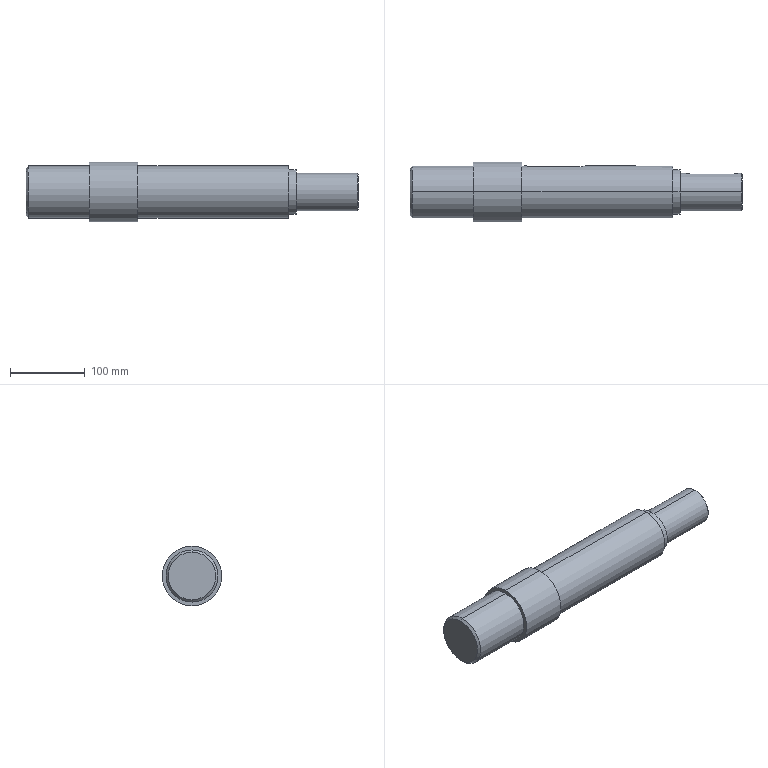Part | SolidWorks | features ICE 6, Chamfer 2, 3DProfileFeature 1, Extrusion 1, RefAxis 1 | 1 solid | 30 faces | box 445 x 80 x 80 mm | volume 1605911 mm3 | cylinder 14 | plane 12 | cone 4 | commonest cylinder face diameters 70 x4 14 x2 20 x2 50 x2 60 x2 80 x2
STEP:
#1=CARTESIAN_POINT('',(360.,0.,-24.));
#2=VERTEX_POINT('',#1);
#3=CARTESIAN_POINT('',(360.,0.,24.));
#4=VERTEX_POINT('',#3);
#5=CARTESIAN_POINT('',(360.,0.,0.));
#6=DIRECTION('',(1.,0.,0.));
#7=DIRECTION('',(0.,0.,-1.));
#8=AXIS2_PLACEMENT_3D('',#5,#6,#7);
#9=CIRCLE('',#8,24.);
#10=EDGE_CURVE('',#2,#4,#9,.T.);
#11=ORIENTED_EDGE('',*,*,#10,.F.);
#12=CARTESIAN_POINT('',(359.,0.,-25.));
#13=VERTEX_POINT('',#12);
#14=CARTESIAN_POINT('',(360.,0.,-24.));
#15=DIRECTION('',(-0.7071,0.,-0.7071));
#16=VECTOR('',#15,1000.);
#17=LINE('',#14,#16);
#18=EDGE_CURVE('',#2,#13,#17,.T.);
#19=ORIENTED_EDGE('',*,*,#18,.T.);
#20=CARTESIAN_POINT('',(359.,0.,25.));
#21=VERTEX_POINT('',#20);
#22=CARTESIAN_POINT('',(359.,0.,0.));
#23=DIRECTION('',(-1.,0.,0.));
#24=DIRECTION('',(0.,0.,-1.));
#25=AXIS2_PLACEMENT_3D('',#22,#23,#24);
#26=CIRCLE('',#25,25.);
#27=EDGE_CURVE('',#21,#13,#26,.T.);
#28=ORIENTED_EDGE('',*,*,#27,.F.);
#29=CARTESIAN_POINT('',(360.,0.,24.));
#30=DIRECTION('',(-0.7071,0.,0.7071));
#31=VECTOR('',#30,1000.);
#32=LINE('',#29,#31);
#33=EDGE_CURVE('',#4,#21,#32,.T.);
#34=ORIENTED_EDGE('',*,*,#33,.F.);
#35=EDGE_LOOP('',(#11,#19,#28,#34));
#36=FACE_OUTER_BOUND('',#35,.T.);
#37=CARTESIAN_POINT('',(360.,0.,0.));
#38=DIRECTION('',(-1.,0.,0.));
#39=DIRECTION('',(0.,0.,1.));
#40=AXIS2_PLACEMENT_3D('',#37,#38,#39);
#41=CONICAL_SURFACE('',#40,24.,0.7854);
#42=ADVANCED_FACE('',(#36),#41,.T.);
#43=CARTESIAN_POINT('',(277.,0.,-30.));
#44=VERTEX_POINT('',#43);
#45=CARTESIAN_POINT('',(277.,0.,30.));
#46=VERTEX_POINT('',#45);
#47=CARTESIAN_POINT('',(277.,0.,0.));
#48=DIRECTION('',(1.,0.,0.));
#49=DIRECTION('',(0.,0.,-1.));
#50=AXIS2_PLACEMENT_3D('',#47,#48,#49);
#51=CIRCLE('',#50,30.);
#52=EDGE_CURVE('',#44,#46,#51,.T.);
#53=ORIENTED_EDGE('',*,*,#52,.F.);
#54=CARTESIAN_POINT('',(267.,0.,-30.));
#55=VERTEX_POINT('',#54);
#56=CARTESIAN_POINT('',(277.,0.,-30.));
#57=DIRECTION('',(-1.,0.,0.));
#58=VECTOR('',#57,1000.);
#59=LINE('',#56,#58);
#60=EDGE_CURVE('',#44,#55,#59,.T.);
#61=ORIENTED_EDGE('',*,*,#60,.T.);
#62=CARTESIAN_POINT('',(267.,0.,30.));
#63=VERTEX_POINT('',#62);
#64=CARTESIAN_POINT('',(267.,0.,0.));
#65=DIRECTION('',(1.,0.,0.));
#66=DIRECTION('',(0.,0.,-1.));
#67=AXIS2_PLACEMENT_3D('',#64,#65,#66);
#68=CIRCLE('',#67,30.);
#69=EDGE_CURVE('',#55,#63,#68,.T.);
#70=ORIENTED_EDGE('',*,*,#69,.T.);
#71=CARTESIAN_POINT('',(277.,0.,30.));
#72=DIRECTION('',(-1.,0.,0.));
#73=VECTOR('',#72,1000.);
#74=LINE('',#71,#73);
#75=EDGE_CURVE('',#46,#63,#74,.T.);
#76=ORIENTED_EDGE('',*,*,#75,.F.);
#77=EDGE_LOOP('',(#53,#61,#70,#76));
#78=FACE_OUTER_BOUND('',#77,.T.);
#79=CARTESIAN_POINT('',(277.,0.,0.));
#80=DIRECTION('',(-1.,0.,0.));
#81=DIRECTION('',(0.,0.,1.));
#82=AXIS2_PLACEMENT_3D('',#79,#80,#81);
#83=CYLINDRICAL_SURFACE('',#82,30.);
#84=ADVANCED_FACE('',(#78),#83,.T.);
#85=CARTESIAN_POINT('',(-85.,0.,32.));
#86=VERTEX_POINT('',#85);
#87=CARTESIAN_POINT('',(-85.,0.,-32.));
#88=VERTEX_POINT('',#87);
#89=CARTESIAN_POINT('',(-85.,0.,0.));
#90=DIRECTION('',(-1.,0.,0.));
#91=DIRECTION('',(0.,0.,1.));
#92=AXIS2_PLACEMENT_3D('',#89,#90,#91);
#93=CIRCLE('',#92,32.);
#94=EDGE_CURVE('',#86,#88,#93,.T.);
#95=ORIENTED_EDGE('',*,*,#94,.F.);
#96=CARTESIAN_POINT('',(-82.,0.,35.));
#97=VERTEX_POINT('',#96);
#98=CARTESIAN_POINT('',(-85.,0.,32.));
#99=DIRECTION('',(0.7071,0.,0.7071));
#100=VECTOR('',#99,1000.);
#101=LINE('',#98,#100);
#102=EDGE_CURVE('',#86,#97,#101,.T.);
#103=ORIENTED_EDGE('',*,*,#102,.T.);
#104=CARTESIAN_POINT('',(-82.,0.,-35.));
#105=VERTEX_POINT('',#104);
#106=CARTESIAN_POINT('',(-82.,0.,0.));
#107=DIRECTION('',(1.,0.,0.));
#108=DIRECTION('',(0.,0.,1.));
#109=AXIS2_PLACEMENT_3D('',#106,#107,#108);
#110=CIRCLE('',#109,35.);
#111=EDGE_CURVE('',#105,#97,#110,.T.);
#112=ORIENTED_EDGE('',*,*,#111,.F.);
#113=CARTESIAN_POINT('',(-85.,0.,-32.));
#114=DIRECTION('',(0.7071,0.,-0.7071));
#115=VECTOR('',#114,1000.);
#116=LINE('',#113,#115);
#117=EDGE_CURVE('',#88,#105,#116,.T.);
#118=ORIENTED_EDGE('',*,*,#117,.F.);
#119=EDGE_LOOP('',(#95,#103,#112,#118));
#120=FACE_OUTER_BOUND('',#119,.T.);
#121=CARTESIAN_POINT('',(-85.,0.,0.));
#122=DIRECTION('',(1.,0.,0.));
#123=DIRECTION('',(0.,0.,-1.));
#124=AXIS2_PLACEMENT_3D('',#121,#122,#123);
#125=CONICAL_SURFACE('',#124,32.,0.7854);
#126=ADVANCED_FACE('',(#120),#125,.T.);
#127=ORIENTED_EDGE('',*,*,#111,.T.);
#128=CARTESIAN_POINT('',(0.,0.,35.));
#129=VERTEX_POINT('',#128);
#130=CARTESIAN_POINT('',(-85.,0.,35.));
#131=DIRECTION('',(1.,0.,0.));
#132=VECTOR('',#131,1000.);
#133=LINE('',#130,#132);
#134=EDGE_CURVE('',#97,#129,#133,.T.);
#135=ORIENTED_EDGE('',*,*,#134,.T.);
#136=CARTESIAN_POINT('',(0.,0.,-35.));
#137=VERTEX_POINT('',#136);
#138=CARTESIAN_POINT('',(0.,0.,0.));
#139=DIRECTION('',(-1.,0.,0.));
#140=DIRECTION('',(0.,0.,-1.));
#141=AXIS2_PLACEMENT_3D('',#138,#139,#140);
#142=CIRCLE('',#141,35.);
#143=EDGE_CURVE('',#129,#137,#142,.T.);
#144=ORIENTED_EDGE('',*,*,#143,.T.);
#145=CARTESIAN_POINT('',(-85.,0.,-35.));
#146=DIRECTION('',(1.,0.,0.));
#147=VECTOR('',#146,1000.);
#148=LINE('',#145,#147);
#149=EDGE_CURVE('',#105,#137,#148,.T.);
#150=ORIENTED_EDGE('',*,*,#149,.F.);
#151=EDGE_LOOP('',(#127,#135,#144,#150));
#152=FACE_OUTER_BOUND('',#151,.T.);
#153=CARTESIAN_POINT('',(-85.,0.,0.));
#154=DIRECTION('',(1.,0.,0.));
#155=DIRECTION('',(0.,0.,-1.));
#156=AXIS2_PLACEMENT_3D('',#153,#154,#155);
#157=CYLINDRICAL_SURFACE('',#156,35.);
#158=ADVANCED_FACE('',(#152),#157,.T.);
#159=CARTESIAN_POINT('',(65.,0.,-40.));
#160=VERTEX_POINT('',#159);
#161=CARTESIAN_POINT('',(65.,0.,40.));
#162=VERTEX_POINT('',#161);
#163=CARTESIAN_POINT('',(65.,0.,0.));
#164=DIRECTION('',(1.,0.,0.));
#165=DIRECTION('',(0.,0.,-1.));
#166=AXIS2_PLACEMENT_3D('',#163,#164,#165);
#167=CIRCLE('',#166,40.);
#168=EDGE_CURVE('',#160,#162,#167,.T.);
#169=ORIENTED_EDGE('',*,*,#168,.F.);
#170=CARTESIAN_POINT('',(0.,0.,-40.));
#171=VERTEX_POINT('',#170);
#172=CARTESIAN_POINT('',(65.,0.,-40.));
#173=DIRECTION('',(-1.,0.,0.));
#174=VECTOR('',#173,1000.);
#175=LINE('',#172,#174);
#176=EDGE_CURVE('',#160,#171,#175,.T.);
#177=ORIENTED_EDGE('',*,*,#176,.T.);
#178=CARTESIAN_POINT('',(0.,0.,40.));
#179=VERTEX_POINT('',#178);
#180=CARTESIAN_POINT('',(0.,0.,0.));
#181=DIRECTION('',(1.,0.,0.));
#182=DIRECTION('',(0.,0.,-1.));
#183=AXIS2_PLACEMENT_3D('',#180,#181,#182);
#184=CIRCLE('',#183,40.);
#185=EDGE_CURVE('',#171,#179,#184,.T.);
#186=ORIENTED_EDGE('',*,*,#185,.T.);
#187=CARTESIAN_POINT('',(65.,0.,40.));
#188=DIRECTION('',(-1.,0.,0.));
#189=VECTOR('',#188,1000.);
#190=LINE('',#187,#189);
#191=EDGE_CURVE('',#162,#179,#190,.T.);
#192=ORIENTED_EDGE('',*,*,#191,.F.);
#193=EDGE_LOOP('',(#169,#177,#186,#192));
#194=FACE_OUTER_BOUND('',#193,.T.);
#195=CARTESIAN_POINT('',(65.,0.,0.));
#196=DIRECTION('',(-1.,0.,0.));
#197=DIRECTION('',(0.,0.,1.));
#198=AXIS2_PLACEMENT_3D('',#195,#196,#197);
#199=CYLINDRICAL_SURFACE('',#198,40.);
#200=ADVANCED_FACE('',(#194),#199,.T.);
#201=CARTESIAN_POINT('',(80.,33.541,-10.));
#202=VERTEX_POINT('',#201);
#203=CARTESIAN_POINT('',(80.,33.541,10.));
#204=VERTEX_POINT('',#203);
#205=CARTESIAN_POINT('',(80.,33.541,-10.));
#206=CARTESIAN_POINT('',(79.336,33.541,-10.));
#207=CARTESIAN_POINT('',(78.683,33.561,-9.934));
#208=CARTESIAN_POINT('',(77.722,33.617,-9.742));
#209=CARTESIAN_POINT('',(77.404,33.64,-9.663));
#210=CARTESIAN_POINT('',(76.774,33.694,-9.471));
#211=CARTESIAN_POINT('',(76.462,33.726,-9.359));
#212=CARTESIAN_POINT('',(75.555,33.829,-8.982));
#213=CARTESIAN_POINT('',(74.982,33.91,-8.675));
#214=CARTESIAN_POINT('',(74.169,34.043,-8.131));
#215=CARTESIAN_POINT('',(73.905,34.089,-7.934));
#216=CARTESIAN_POINT('',(73.399,34.183,-7.519));
#217=CARTESIAN_POINT('',(73.159,34.231,-7.301));
#218=CARTESIAN_POINT('',(72.471,34.373,-6.613));
#219=CARTESIAN_POINT('',(72.058,34.467,-6.112));
#220=CARTESIAN_POINT('',(71.327,34.642,-5.02));
#221=CARTESIAN_POINT('',(71.018,34.722,-4.444));
#222=CARTESIAN_POINT('',(70.643,34.822,-3.543));
#223=CARTESIAN_POINT('',(70.532,34.852,-3.236));
#224=CARTESIAN_POINT('',(70.341,34.904,-2.608));
#225=CARTESIAN_POINT('',(70.259,34.927,-2.286));
#226=CARTESIAN_POINT('',(70.065,34.981,-1.317));
#227=CARTESIAN_POINT('',(70.001,35.,-0.6655));
#228=CARTESIAN_POINT('',(69.999,35.,0.6464));
#229=CARTESIAN_POINT('',(70.065,34.981,1.313));
#230=CARTESIAN_POINT('',(70.321,34.909,2.598));
#231=CARTESIAN_POINT('',(70.511,34.857,3.223));
#232=CARTESIAN_POINT('',(70.889,34.756,4.135));
#233=CARTESIAN_POINT('',(71.031,34.719,4.433));
#234=CARTESIAN_POINT('',(71.339,34.641,5.009));
#235=CARTESIAN_POINT('',(71.506,34.599,5.288));
#236=CARTESIAN_POINT('',(71.867,34.512,5.828));
#237=CARTESIAN_POINT('',(72.061,34.467,6.089));
#238=CARTESIAN_POINT('',(72.474,34.374,6.593));
#239=CARTESIAN_POINT('',(72.696,34.326,6.838));
#240=CARTESIAN_POINT('',(73.388,34.183,7.531));
#241=CARTESIAN_POINT('',(73.889,34.089,7.942));
#242=CARTESIAN_POINT('',(74.969,33.912,8.666));
#243=CARTESIAN_POINT('',(75.554,33.829,8.981));
#244=CARTESIAN_POINT('',(76.759,33.692,9.483));
#245=CARTESIAN_POINT('',(77.382,33.637,9.674));
#246=CARTESIAN_POINT('',(78.349,33.58,9.868));
#247=CARTESIAN_POINT('',(78.678,33.565,9.918));
#248=CARTESIAN_POINT('',(79.337,33.546,9.983));
#249=CARTESIAN_POINT('',(79.668,33.541,10.));
#250=CARTESIAN_POINT('',(80.,33.541,10.));
#251=B_SPLINE_CURVE_WITH_KNOTS('',3,(#205,#206,#207,#208,#209,#210,#211,#212,#213,#214,#215,#216,#217,#218,#219,#220,#221,#222,#223,#224,#225,#226,#227,#228,#229,#230,#231,#232,#233,#234,#235,#236,#237,#238,#239,#240,#241,#242,#243,#244,#245,#246,#247,#248,#249,#250),.UNSPECIFIED.,.F.,.F.,(4,2,2,2,2,2,2,2,2,2,2,2,2,2,2,2,2,2,2,2,2,2,4),(0.,0.001964,0.002945,0.003927,0.005891,0.006873,0.007855,0.009818,0.01178,0.01276,0.01375,0.01571,0.01767,0.01964,0.02062,0.0216,0.02258,0.02356,0.02553,0.02749,0.02945,0.03044,0.03142),.UNSPECIFIED.);
#252=EDGE_CURVE('',#202,#204,#251,.T.);
#253=ORIENTED_EDGE('',*,*,#252,.F.);
#254=CARTESIAN_POINT('',(140.,33.541,-10.));
#255=VERTEX_POINT('',#254);
#256=CARTESIAN_POINT('',(267.,33.541,-10.));
#257=DIRECTION('',(-1.,0.,0.));
#258=VECTOR('',#257,1000.);
#259=LINE('',#256,#258);
#260=EDGE_CURVE('',#255,#202,#259,.T.);
#261=ORIENTED_EDGE('',*,*,#260,.F.);
#262=CARTESIAN_POINT('',(140.,33.541,10.));
#263=VERTEX_POINT('',#262);
#264=CARTESIAN_POINT('',(140.,33.541,10.));
#265=CARTESIAN_POINT('',(140.664,33.541,10.));
#266=CARTESIAN_POINT('',(141.317,33.561,9.934));
#267=CARTESIAN_POINT('',(142.278,33.617,9.742));
#268=CARTESIAN_POINT('',(142.596,33.64,9.663));
#269=CARTESIAN_POINT('',(143.226,33.694,9.471));
#270=CARTESIAN_POINT('',(143.538,33.726,9.359));
#271=CARTESIAN_POINT('',(144.445,33.829,8.982));
#272=CARTESIAN_POINT('',(145.018,33.91,8.675));
#273=CARTESIAN_POINT('',(145.831,34.043,8.131));
#274=CARTESIAN_POINT('',(146.095,34.089,7.934));
#275=CARTESIAN_POINT('',(146.601,34.183,7.519));
#276=CARTESIAN_POINT('',(146.841,34.231,7.301));
#277=CARTESIAN_POINT('',(147.529,34.373,6.613));
#278=CARTESIAN_POINT('',(147.942,34.467,6.112));
#279=CARTESIAN_POINT('',(148.673,34.642,5.02));
#280=CARTESIAN_POINT('',(148.982,34.722,4.444));
#281=CARTESIAN_POINT('',(149.357,34.822,3.543));
#282=CARTESIAN_POINT('',(149.468,34.852,3.236));
#283=CARTESIAN_POINT('',(149.659,34.904,2.608));
#284=CARTESIAN_POINT('',(149.741,34.927,2.286));
#285=CARTESIAN_POINT('',(149.935,34.981,1.317));
#286=CARTESIAN_POINT('',(149.999,35.,0.6655));
#287=CARTESIAN_POINT('',(150.001,35.,-0.6464));
#288=CARTESIAN_POINT('',(149.935,34.981,-1.313));
#289=CARTESIAN_POINT('',(149.679,34.909,-2.598));
#290=CARTESIAN_POINT('',(149.489,34.857,-3.223));
#291=CARTESIAN_POINT('',(149.111,34.756,-4.135));
#292=CARTESIAN_POINT('',(148.969,34.719,-4.433));
#293=CARTESIAN_POINT('',(148.661,34.641,-5.009));
#294=CARTESIAN_POINT('',(148.494,34.599,-5.288));
#295=CARTESIAN_POINT('',(148.133,34.512,-5.828));
#296=CARTESIAN_POINT('',(147.939,34.467,-6.089));
#297=CARTESIAN_POINT('',(147.526,34.374,-6.593));
#298=CARTESIAN_POINT('',(147.304,34.326,-6.838));
#299=CARTESIAN_POINT('',(146.612,34.183,-7.531));
#300=CARTESIAN_POINT('',(146.111,34.089,-7.942));
#301=CARTESIAN_POINT('',(145.031,33.912,-8.666));
#302=CARTESIAN_POINT('',(144.446,33.829,-8.981));
#303=CARTESIAN_POINT('',(143.241,33.692,-9.483));
#304=CARTESIAN_POINT('',(142.618,33.637,-9.674));
#305=CARTESIAN_POINT('',(141.651,33.58,-9.868));
#306=CARTESIAN_POINT('',(141.322,33.565,-9.918));
#307=CARTESIAN_POINT('',(140.663,33.546,-9.983));
#308=CARTESIAN_POINT('',(140.332,33.541,-10.));
#309=CARTESIAN_POINT('',(140.,33.541,-10.));
#310=B_SPLINE_CURVE_WITH_KNOTS('',3,(#264,#265,#266,#267,#268,#269,#270,#271,#272,#273,#274,#275,#276,#277,#278,#279,#280,#281,#282,#283,#284,#285,#286,#287,#288,#289,#290,#291,#292,#293,#294,#295,#296,#297,#298,#299,#300,#301,#302,#303,#304,#305,#306,#307,#308,#309),.UNSPECIFIED.,.F.,.F.,(4,2,2,2,2,2,2,2,2,2,2,2,2,2,2,2,2,2,2,2,2,2,4),(0.,0.001964,0.002945,0.003927,0.005891,0.006873,0.007855,0.009818,0.01178,0.01276,0.01375,0.01571,0.01767,0.01964,0.02062,0.0216,0.02258,0.02356,0.02553,0.02749,0.02945,0.03044,0.03142),.UNSPECIFIED.);
#311=EDGE_CURVE('',#263,#255,#310,.T.);
#312=ORIENTED_EDGE('',*,*,#311,.F.);
#313=CARTESIAN_POINT('',(267.,33.541,10.));
#314=DIRECTION('',(1.,0.,0.));
#315=VECTOR('',#314,1000.);
#316=LINE('',#313,#315);
#317=EDGE_CURVE('',#204,#263,#316,.T.);
#318=ORIENTED_EDGE('',*,*,#317,.F.);
#319=EDGE_LOOP('',(#253,#261,#312,#318));
#320=FACE_BOUND('',#319,.T.);
#321=CARTESIAN_POINT('',(267.,0.,-35.));
#322=VERTEX_POINT('',#321);
#323=CARTESIAN_POINT('',(267.,0.,35.));
#324=VERTEX_POINT('',#323);
#325=CARTESIAN_POINT('',(267.,0.,0.));
#326=DIRECTION('',(1.,0.,0.));
#327=DIRECTION('',(0.,0.,-1.));
#328=AXIS2_PLACEMENT_3D('',#325,#326,#327);
#329=CIRCLE('',#328,35.);
#330=EDGE_CURVE('',#322,#324,#329,.T.);
#331=ORIENTED_EDGE('',*,*,#330,.F.);
#332=CARTESIAN_POINT('',(65.,0.,-35.));
#333=VERTEX_POINT('',#332);
#334=CARTESIAN_POINT('',(267.,0.,-35.));
#335=DIRECTION('',(-1.,0.,0.));
#336=VECTOR('',#335,1000.);
#337=LINE('',#334,#336);
#338=EDGE_CURVE('',#322,#333,#337,.T.);
#339=ORIENTED_EDGE('',*,*,#338,.T.);
#340=CARTESIAN_POINT('',(65.,0.,35.));
#341=VERTEX_POINT('',#340);
#342=CARTESIAN_POINT('',(65.,0.,0.));
#343=DIRECTION('',(1.,0.,0.));
#344=DIRECTION('',(0.,0.,-1.));
#345=AXIS2_PLACEMENT_3D('',#342,#343,#344);
#346=CIRCLE('',#345,35.);
#347=EDGE_CURVE('',#333,#341,#346,.T.);
#348=ORIENTED_EDGE('',*,*,#347,.T.);
#349=CARTESIAN_POINT('',(267.,0.,35.));
#350=DIRECTION('',(-1.,0.,0.));
#351=VECTOR('',#350,1000.);
#352=LINE('',#349,#351);
#353=EDGE_CURVE('',#324,#341,#352,.T.);
#354=ORIENTED_EDGE('',*,*,#353,.F.);
#355=EDGE_LOOP('',(#331,#339,#348,#354));
#356=FACE_OUTER_BOUND('',#355,.T.);
#357=CARTESIAN_POINT('',(267.,0.,0.));
#358=DIRECTION('',(-1.,0.,0.));
#359=DIRECTION('',(0.,0.,1.));
#360=AXIS2_PLACEMENT_3D('',#357,#358,#359);
#361=CYLINDRICAL_SURFACE('',#360,35.);
#362=ADVANCED_FACE('',(#320,#356),#361,.T.);
#363=CARTESIAN_POINT('',(292.,24.,-7.));
#364=VERTEX_POINT('',#363);
#365=CARTESIAN_POINT('',(292.,24.,7.));
#366=VERTEX_POINT('',#365);
#367=CARTESIAN_POINT('',(292.,24.,-7.));
#368=CARTESIAN_POINT('',(291.535,24.,-7.));
#369=CARTESIAN_POINT('',(291.079,24.014,-6.954));
#370=CARTESIAN_POINT('',(290.405,24.052,-6.82));
#371=CARTESIAN_POINT('',(290.183,24.068,-6.764));
#372=CARTESIAN_POINT('',(289.742,24.105,-6.63));
#373=CARTESIAN_POINT('',(289.524,24.126,-6.551));
#374=CARTESIAN_POINT('',(288.889,24.197,-6.287));
#375=CARTESIAN_POINT('',(288.488,24.253,-6.072));
#376=CARTESIAN_POINT('',(287.919,24.344,-5.692));
#377=CARTESIAN_POINT('',(287.733,24.376,-5.554));
#378=CARTESIAN_POINT('',(287.38,24.44,-5.263));
#379=CARTESIAN_POINT('',(287.211,24.473,-5.11));
#380=CARTESIAN_POINT('',(286.729,24.57,-4.629));
#381=CARTESIAN_POINT('',(286.44,24.634,-4.278));
#382=CARTESIAN_POINT('',(285.929,24.755,-3.514));
#383=CARTESIAN_POINT('',(285.713,24.809,-3.11));
#384=CARTESIAN_POINT('',(285.45,24.878,-2.48));
#385=CARTESIAN_POINT('',(285.373,24.898,-2.265));
#386=CARTESIAN_POINT('',(285.238,24.934,-1.825));
#387=CARTESIAN_POINT('',(285.181,24.95,-1.6));
#388=CARTESIAN_POINT('',(285.046,24.987,-0.9213));
#389=CARTESIAN_POINT('',(285.,25.,-0.4657));
#390=CARTESIAN_POINT('',(285.,25.,0.4524));
#391=CARTESIAN_POINT('',(285.045,24.987,0.9188));
#392=CARTESIAN_POINT('',(285.225,24.938,1.818));
#393=CARTESIAN_POINT('',(285.358,24.902,2.256));
#394=CARTESIAN_POINT('',(285.622,24.833,2.894));
#395=CARTESIAN_POINT('',(285.721,24.808,3.103));
#396=CARTESIAN_POINT('',(285.937,24.754,3.506));
#397=CARTESIAN_POINT('',(286.054,24.725,3.701));
#398=CARTESIAN_POINT('',(286.307,24.666,4.079));
#399=CARTESIAN_POINT('',(286.442,24.635,4.262));
#400=CARTESIAN_POINT('',(286.732,24.571,4.615));
#401=CARTESIAN_POINT('',(286.887,24.538,4.786));
#402=CARTESIAN_POINT('',(287.372,24.44,5.272));
#403=CARTESIAN_POINT('',(287.722,24.375,5.56));
#404=CARTESIAN_POINT('',(288.478,24.254,6.067));
#405=CARTESIAN_POINT('',(288.888,24.197,6.287));
#406=CARTESIAN_POINT('',(289.731,24.103,6.638));
#407=CARTESIAN_POINT('',(290.168,24.066,6.772));
#408=CARTESIAN_POINT('',(290.844,24.027,6.908));
#409=CARTESIAN_POINT('',(291.075,24.017,6.942));
#410=CARTESIAN_POINT('',(291.536,24.003,6.988));
#411=CARTESIAN_POINT('',(291.768,24.,7.));
#412=CARTESIAN_POINT('',(292.,24.,7.));
#413=B_SPLINE_CURVE_WITH_KNOTS('',3,(#367,#368,#369,#370,#371,#372,#373,#374,#375,#376,#377,#378,#379,#380,#381,#382,#383,#384,#385,#386,#387,#388,#389,#390,#391,#392,#393,#394,#395,#396,#397,#398,#399,#400,#401,#402,#403,#404,#405,#406,#407,#408,#409,#410,#411,#412),.UNSPECIFIED.,.F.,.F.,(4,2,2,2,2,2,2,2,2,2,2,2,2,2,2,2,2,2,2,2,2,2,4),(0.,0.001374,0.002061,0.002749,0.004123,0.00481,0.005497,0.006871,0.008246,0.008933,0.00962,0.01099,0.01237,0.01374,0.01443,0.01512,0.0158,0.01649,0.01787,0.01924,0.02061,0.0213,0.02199),.UNSPECIFIED.);
#414=EDGE_CURVE('',#364,#366,#413,.T.);
#415=ORIENTED_EDGE('',*,*,#414,.F.);
#416=CARTESIAN_POINT('',(348.,24.,-7.));
#417=VERTEX_POINT('',#416);
#418=CARTESIAN_POINT('',(360.,24.,-7.));
#419=DIRECTION('',(-1.,0.,0.));
#420=VECTOR('',#419,1000.);
#421=LINE('',#418,#420);
#422=EDGE_CURVE('',#417,#364,#421,.T.);
#423=ORIENTED_EDGE('',*,*,#422,.F.);
#424=CARTESIAN_POINT('',(348.,24.,7.));
#425=VERTEX_POINT('',#424);
#426=CARTESIAN_POINT('',(348.,24.,7.));
#427=CARTESIAN_POINT('',(348.465,24.,7.));
#428=CARTESIAN_POINT('',(348.921,24.014,6.954));
#429=CARTESIAN_POINT('',(349.595,24.052,6.82));
#430=CARTESIAN_POINT('',(349.817,24.068,6.764));
#431=CARTESIAN_POINT('',(350.258,24.105,6.63));
#432=CARTESIAN_POINT('',(350.476,24.126,6.551));
#433=CARTESIAN_POINT('',(351.111,24.197,6.287));
#434=CARTESIAN_POINT('',(351.512,24.253,6.072));
#435=CARTESIAN_POINT('',(352.081,24.344,5.692));
#436=CARTESIAN_POINT('',(352.267,24.376,5.554));
#437=CARTESIAN_POINT('',(352.62,24.44,5.263));
#438=CARTESIAN_POINT('',(352.789,24.473,5.11));
#439=CARTESIAN_POINT('',(353.271,24.57,4.629));
#440=CARTESIAN_POINT('',(353.56,24.634,4.278));
#441=CARTESIAN_POINT('',(354.071,24.755,3.514));
#442=CARTESIAN_POINT('',(354.287,24.809,3.11));
#443=CARTESIAN_POINT('',(354.55,24.878,2.48));
#444=CARTESIAN_POINT('',(354.627,24.898,2.265));
#445=CARTESIAN_POINT('',(354.762,24.934,1.825));
#446=CARTESIAN_POINT('',(354.819,24.95,1.6));
#447=CARTESIAN_POINT('',(354.954,24.987,0.9213));
#448=CARTESIAN_POINT('',(355.,25.,0.4657));
#449=CARTESIAN_POINT('',(355.,25.,-0.4524));
#450=CARTESIAN_POINT('',(354.955,24.987,-0.9188));
#451=CARTESIAN_POINT('',(354.775,24.938,-1.818));
#452=CARTESIAN_POINT('',(354.642,24.902,-2.256));
#453=CARTESIAN_POINT('',(354.378,24.833,-2.894));
#454=CARTESIAN_POINT('',(354.279,24.808,-3.103));
#455=CARTESIAN_POINT('',(354.063,24.754,-3.506));
#456=CARTESIAN_POINT('',(353.946,24.725,-3.701));
#457=CARTESIAN_POINT('',(353.693,24.666,-4.079));
#458=CARTESIAN_POINT('',(353.558,24.635,-4.262));
#459=CARTESIAN_POINT('',(353.268,24.571,-4.615));
#460=CARTESIAN_POINT('',(353.113,24.538,-4.786));
#461=CARTESIAN_POINT('',(352.628,24.44,-5.272));
#462=CARTESIAN_POINT('',(352.278,24.375,-5.56));
#463=CARTESIAN_POINT('',(351.522,24.254,-6.067));
#464=CARTESIAN_POINT('',(351.112,24.197,-6.287));
#465=CARTESIAN_POINT('',(350.269,24.103,-6.638));
#466=CARTESIAN_POINT('',(349.832,24.066,-6.772));
#467=CARTESIAN_POINT('',(349.156,24.027,-6.908));
#468=CARTESIAN_POINT('',(348.925,24.017,-6.942));
#469=CARTESIAN_POINT('',(348.464,24.003,-6.988));
#470=CARTESIAN_POINT('',(348.232,24.,-7.));
#471=CARTESIAN_POINT('',(348.,24.,-7.));
#472=B_SPLINE_CURVE_WITH_KNOTS('',3,(#426,#427,#428,#429,#430,#431,#432,#433,#434,#435,#436,#437,#438,#439,#440,#441,#442,#443,#444,#445,#446,#447,#448,#449,#450,#451,#452,#453,#454,#455,#456,#457,#458,#459,#460,#461,#462,#463,#464,#465,#466,#467,#468,#469,#470,#471),.UNSPECIFIED.,.F.,.F.,(4,2,2,2,2,2,2,2,2,2,2,2,2,2,2,2,2,2,2,2,2,2,4),(0.,0.001374,0.002061,0.002749,0.004123,0.00481,0.005497,0.006871,0.008246,0.008933,0.00962,0.01099,0.01237,0.01374,0.01443,0.01512,0.0158,0.01649,0.01787,0.01924,0.02061,0.0213,0.02199),.UNSPECIFIED.);
#473=EDGE_CURVE('',#425,#417,#472,.T.);
#474=ORIENTED_EDGE('',*,*,#473,.F.);
#475=CARTESIAN_POINT('',(360.,24.,7.));
#476=DIRECTION('',(1.,0.,0.));
#477=VECTOR('',#476,1000.);
#478=LINE('',#475,#477);
#479=EDGE_CURVE('',#366,#425,#478,.T.);
#480=ORIENTED_EDGE('',*,*,#479,.F.);
#481=EDGE_LOOP('',(#415,#423,#474,#480));
#482=FACE_BOUND('',#481,.T.);
#483=ORIENTED_EDGE('',*,*,#27,.T.);
#484=CARTESIAN_POINT('',(277.,0.,-25.));
#485=VERTEX_POINT('',#484);
#486=CARTESIAN_POINT('',(360.,0.,-25.));
#487=DIRECTION('',(-1.,0.,0.));
#488=VECTOR('',#487,1000.);
#489=LINE('',#486,#488);
#490=EDGE_CURVE('',#13,#485,#489,.T.);
#491=ORIENTED_EDGE('',*,*,#490,.T.);
#492=CARTESIAN_POINT('',(277.,0.,25.));
#493=VERTEX_POINT('',#492);
#494=CARTESIAN_POINT('',(277.,0.,0.));
#495=DIRECTION('',(1.,0.,0.));
#496=DIRECTION('',(0.,0.,-1.));
#497=AXIS2_PLACEMENT_3D('',#494,#495,#496);
#498=CIRCLE('',#497,25.);
#499=EDGE_CURVE('',#485,#493,#498,.T.);
#500=ORIENTED_EDGE('',*,*,#499,.T.);
#501=CARTESIAN_POINT('',(360.,0.,25.));
#502=DIRECTION('',(-1.,0.,0.));
#503=VECTOR('',#502,1000.);
#504=LINE('',#501,#503);
#505=EDGE_CURVE('',#21,#493,#504,.T.);
#506=ORIENTED_EDGE('',*,*,#505,.F.);
#507=EDGE_LOOP('',(#483,#491,#500,#506));
#508=FACE_OUTER_BOUND('',#507,.T.);
#509=CARTESIAN_POINT('',(360.,0.,0.));
#510=DIRECTION('',(-1.,0.,0.));
#511=DIRECTION('',(0.,0.,1.));
#512=AXIS2_PLACEMENT_3D('',#509,#510,#511);
#513=CYLINDRICAL_SURFACE('',#512,25.);
#514=ADVANCED_FACE('',(#482,#508),#513,.T.);
#515=ORIENTED_EDGE('',*,*,#490,.F.);
#516=CARTESIAN_POINT('',(359.,0.,0.));
#517=DIRECTION('',(-1.,0.,0.));
#518=DIRECTION('',(0.,0.,-1.));
#519=AXIS2_PLACEMENT_3D('',#516,#517,#518);
#520=CIRCLE('',#519,25.);
#521=EDGE_CURVE('',#13,#21,#520,.T.);
#522=ORIENTED_EDGE('',*,*,#521,.T.);
#523=ORIENTED_EDGE('',*,*,#505,.T.);
#524=CARTESIAN_POINT('',(277.,0.,0.));
#525=DIRECTION('',(1.,0.,0.));
#526=DIRECTION('',(0.,0.,-1.));
#527=AXIS2_PLACEMENT_3D('',#524,#525,#526);
#528=CIRCLE('',#527,25.);
#529=EDGE_CURVE('',#493,#485,#528,.T.);
#530=ORIENTED_EDGE('',*,*,#529,.T.);
#531=EDGE_LOOP('',(#515,#522,#523,#530));
#532=FACE_OUTER_BOUND('',#531,.T.);
#533=CARTESIAN_POINT('',(360.,0.,0.));
#534=DIRECTION('',(-1.,0.,0.));
#535=DIRECTION('',(0.,0.,1.));
#536=AXIS2_PLACEMENT_3D('',#533,#534,#535);
#537=CYLINDRICAL_SURFACE('',#536,25.);
#538=ADVANCED_FACE('',(#532),#537,.T.);
#539=CARTESIAN_POINT('',(277.,0.,0.));
#540=DIRECTION('',(1.,0.,0.));
#541=DIRECTION('',(0.,0.,-1.));
#542=AXIS2_PLACEMENT_3D('',#539,#540,#541);
#543=CIRCLE('',#542,30.);
#544=EDGE_CURVE('',#46,#44,#543,.T.);
#545=ORIENTED_EDGE('',*,*,#544,.T.);
#546=ORIENTED_EDGE('',*,*,#52,.T.);
#547=EDGE_LOOP('',(#545,#546));
#548=FACE_OUTER_BOUND('',#547,.T.);
#549=ORIENTED_EDGE('',*,*,#529,.F.);
#550=ORIENTED_EDGE('',*,*,#499,.F.);
#551=EDGE_LOOP('',(#549,#550));
#552=FACE_BOUND('',#551,.T.);
#553=CARTESIAN_POINT('',(277.,0.,0.));
#554=DIRECTION('',(1.,0.,0.));
#555=DIRECTION('',(0.,0.,-1.));
#556=AXIS2_PLACEMENT_3D('',#553,#554,#555);
#557=PLANE('',#556);
#558=ADVANCED_FACE('',(#548,#552),#557,.T.);
#559=CARTESIAN_POINT('',(267.,0.,0.));
#560=DIRECTION('',(1.,0.,0.));
#561=DIRECTION('',(0.,0.,-1.));
#562=AXIS2_PLACEMENT_3D('',#559,#560,#561);
#563=CIRCLE('',#562,35.);
#564=EDGE_CURVE('',#324,#322,#563,.T.);
#565=ORIENTED_EDGE('',*,*,#564,.T.);
#566=ORIENTED_EDGE('',*,*,#330,.T.);
#567=EDGE_LOOP('',(#565,#566));
#568=FACE_OUTER_BOUND('',#567,.T.);
#569=CARTESIAN_POINT('',(267.,0.,0.));
#570=DIRECTION('',(1.,0.,0.));
#571=DIRECTION('',(0.,0.,-1.));
#572=AXIS2_PLACEMENT_3D('',#569,#570,#571);
#573=CIRCLE('',#572,30.);
#574=EDGE_CURVE('',#63,#55,#573,.T.);
#575=ORIENTED_EDGE('',*,*,#574,.F.);
#576=ORIENTED_EDGE('',*,*,#69,.F.);
#577=EDGE_LOOP('',(#575,#576));
#578=FACE_BOUND('',#577,.T.);
#579=CARTESIAN_POINT('',(267.,0.,0.));
#580=DIRECTION('',(1.,0.,0.));
#581=DIRECTION('',(0.,0.,-1.));
#582=AXIS2_PLACEMENT_3D('',#579,#580,#581);
#583=PLANE('',#582);
#584=ADVANCED_FACE('',(#568,#578),#583,.T.);
#585=ORIENTED_EDGE('',*,*,#338,.F.);
#586=ORIENTED_EDGE('',*,*,#564,.F.);
#587=ORIENTED_EDGE('',*,*,#353,.T.);
#588=CARTESIAN_POINT('',(65.,0.,0.));
#589=DIRECTION('',(1.,0.,0.));
#590=DIRECTION('',(0.,0.,-1.));
#591=AXIS2_PLACEMENT_3D('',#588,#589,#590);
#592=CIRCLE('',#591,35.);
#593=EDGE_CURVE('',#341,#333,#592,.T.);
#594=ORIENTED_EDGE('',*,*,#593,.T.);
#595=EDGE_LOOP('',(#585,#586,#587,#594));
#596=FACE_OUTER_BOUND('',#595,.T.);
#597=CARTESIAN_POINT('',(267.,0.,0.));
#598=DIRECTION('',(-1.,0.,0.));
#599=DIRECTION('',(0.,0.,1.));
#600=AXIS2_PLACEMENT_3D('',#597,#598,#599);
#601=CYLINDRICAL_SURFACE('',#600,35.);
#602=ADVANCED_FACE('',(#596),#601,.T.);
#603=CARTESIAN_POINT('',(0.,0.,0.));
#604=DIRECTION('',(1.,0.,0.));
#605=DIRECTION('',(0.,0.,-1.));
#606=AXIS2_PLACEMENT_3D('',#603,#604,#605);
#607=CIRCLE('',#606,40.);
#608=EDGE_CURVE('',#179,#171,#607,.T.);
#609=ORIENTED_EDGE('',*,*,#608,.F.);
#610=ORIENTED_EDGE('',*,*,#185,.F.);
#611=EDGE_LOOP('',(#609,#610));
#612=FACE_OUTER_BOUND('',#611,.T.);
#613=CARTESIAN_POINT('',(0.,0.,0.));
#614=DIRECTION('',(-1.,0.,0.));
#615=DIRECTION('',(0.,0.,-1.));
#616=AXIS2_PLACEMENT_3D('',#613,#614,#615);
#617=CIRCLE('',#616,35.);
#618=EDGE_CURVE('',#137,#129,#617,.T.);
#619=ORIENTED_EDGE('',*,*,#618,.F.);
#620=ORIENTED_EDGE('',*,*,#143,.F.);
#621=EDGE_LOOP('',(#619,#620));
#622=FACE_BOUND('',#621,.T.);
#623=CARTESIAN_POINT('',(0.,0.,0.));
#624=DIRECTION('',(1.,0.,0.));
#625=DIRECTION('',(0.,0.,-1.));
#626=AXIS2_PLACEMENT_3D('',#623,#624,#625);
#627=PLANE('',#626);
#628=ADVANCED_FACE('',(#612,#622),#627,.F.);
#629=CARTESIAN_POINT('',(65.,0.,0.));
#630=DIRECTION('',(1.,0.,0.));
#631=DIRECTION('',(0.,0.,-1.));
#632=AXIS2_PLACEMENT_3D('',#629,#630,#631);
#633=CIRCLE('',#632,40.);
#634=EDGE_CURVE('',#162,#160,#633,.T.);
#635=ORIENTED_EDGE('',*,*,#634,.T.);
#636=ORIENTED_EDGE('',*,*,#168,.T.);
#637=EDGE_LOOP('',(#635,#636));
#638=FACE_OUTER_BOUND('',#637,.T.);
#639=ORIENTED_EDGE('',*,*,#593,.F.);
#640=ORIENTED_EDGE('',*,*,#347,.F.);
#641=EDGE_LOOP('',(#639,#640));
#642=FACE_BOUND('',#641,.T.);
#643=CARTESIAN_POINT('',(65.,0.,0.));
#644=DIRECTION('',(1.,0.,0.));
#645=DIRECTION('',(0.,0.,-1.));
#646=AXIS2_PLACEMENT_3D('',#643,#644,#645);
#647=PLANE('',#646);
#648=ADVANCED_FACE('',(#638,#642),#647,.T.);
#649=ORIENTED_EDGE('',*,*,#176,.F.);
#650=ORIENTED_EDGE('',*,*,#634,.F.);
#651=ORIENTED_EDGE('',*,*,#191,.T.);
#652=ORIENTED_EDGE('',*,*,#608,.T.);
#653=EDGE_LOOP('',(#649,#650,#651,#652));
#654=FACE_OUTER_BOUND('',#653,.T.);
#655=CARTESIAN_POINT('',(65.,0.,0.));
#656=DIRECTION('',(-1.,0.,0.));
#657=DIRECTION('',(0.,0.,1.));
#658=AXIS2_PLACEMENT_3D('',#655,#656,#657);
#659=CYLINDRICAL_SURFACE('',#658,40.);
#660=ADVANCED_FACE('',(#654),#659,.T.);
#661=ORIENTED_EDGE('',*,*,#134,.F.);
#662=CARTESIAN_POINT('',(-82.,0.,0.));
#663=DIRECTION('',(1.,0.,0.));
#664=DIRECTION('',(0.,0.,1.));
#665=AXIS2_PLACEMENT_3D('',#662,#663,#664);
#666=CIRCLE('',#665,35.);
#667=EDGE_CURVE('',#97,#105,#666,.T.);
#668=ORIENTED_EDGE('',*,*,#667,.T.);
#669=ORIENTED_EDGE('',*,*,#149,.T.);
#670=ORIENTED_EDGE('',*,*,#618,.T.);
#671=EDGE_LOOP('',(#661,#668,#669,#670));
#672=FACE_OUTER_BOUND('',#671,.T.);
#673=CARTESIAN_POINT('',(-85.,0.,0.));
#674=DIRECTION('',(1.,0.,0.));
#675=DIRECTION('',(0.,0.,-1.));
#676=AXIS2_PLACEMENT_3D('',#673,#674,#675);
#677=CYLINDRICAL_SURFACE('',#676,35.);
#678=ADVANCED_FACE('',(#672),#677,.T.);
#679=CARTESIAN_POINT('',(-85.,0.,0.));
#680=DIRECTION('',(-1.,0.,0.));
#681=DIRECTION('',(0.,0.,1.));
#682=AXIS2_PLACEMENT_3D('',#679,#680,#681);
#683=CIRCLE('',#682,32.);
#684=EDGE_CURVE('',#88,#86,#683,.T.);
#685=ORIENTED_EDGE('',*,*,#684,.T.);
#686=ORIENTED_EDGE('',*,*,#94,.T.);
#687=EDGE_LOOP('',(#685,#686));
#688=FACE_OUTER_BOUND('',#687,.T.);
#689=CARTESIAN_POINT('',(-85.,0.,0.));
#690=DIRECTION('',(-1.,0.,0.));
#691=DIRECTION('',(0.,0.,1.));
#692=AXIS2_PLACEMENT_3D('',#689,#690,#691);
#693=PLANE('',#692);
#694=ADVANCED_FACE('',(#688),#693,.T.);
#695=ORIENTED_EDGE('',*,*,#102,.F.);
#696=ORIENTED_EDGE('',*,*,#684,.F.);
#697=ORIENTED_EDGE('',*,*,#117,.T.);
#698=ORIENTED_EDGE('',*,*,#667,.F.);
#699=EDGE_LOOP('',(#695,#696,#697,#698));
#700=FACE_OUTER_BOUND('',#699,.T.);
#701=CARTESIAN_POINT('',(-85.,0.,0.));
#702=DIRECTION('',(1.,0.,0.));
#703=DIRECTION('',(0.,0.,-1.));
#704=AXIS2_PLACEMENT_3D('',#701,#702,#703);
#705=CONICAL_SURFACE('',#704,32.,0.7854);
#706=ADVANCED_FACE('',(#700),#705,.T.);
#707=CARTESIAN_POINT('',(140.,27.5,10.));
#708=VERTEX_POINT('',#707);
#709=CARTESIAN_POINT('',(140.,35.,10.));
#710=DIRECTION('',(0.,-1.,0.));
#711=VECTOR('',#710,1000.);
#712=LINE('',#709,#711);
#713=EDGE_CURVE('',#263,#708,#712,.T.);
#714=ORIENTED_EDGE('',*,*,#713,.F.);
#715=ORIENTED_EDGE('',*,*,#311,.T.);
#716=CARTESIAN_POINT('',(140.,27.5,-10.));
#717=VERTEX_POINT('',#716);
#718=CARTESIAN_POINT('',(140.,35.,-10.));
#719=DIRECTION('',(0.,-1.,0.));
#720=VECTOR('',#719,1000.);
#721=LINE('',#718,#720);
#722=EDGE_CURVE('',#255,#717,#721,.T.);
#723=ORIENTED_EDGE('',*,*,#722,.T.);
#724=CARTESIAN_POINT('',(140.,27.5,0.));
#725=DIRECTION('',(0.,1.,0.));
#726=DIRECTION('',(0.,0.,-1.));
#727=AXIS2_PLACEMENT_3D('',#724,#725,#726);
#728=CIRCLE('',#727,10.);
#729=EDGE_CURVE('',#708,#717,#728,.T.);
#730=ORIENTED_EDGE('',*,*,#729,.F.);
#731=EDGE_LOOP('',(#714,#715,#723,#730));
#732=FACE_OUTER_BOUND('',#731,.T.);
#733=CARTESIAN_POINT('',(140.,35.,0.));
#734=DIRECTION('',(0.,-1.,0.));
#735=DIRECTION('',(0.,0.,-1.));
#736=AXIS2_PLACEMENT_3D('',#733,#734,#735);
#737=CYLINDRICAL_SURFACE('',#736,10.);
#738=ADVANCED_FACE('',(#732),#737,.F.);
#739=ORIENTED_EDGE('',*,*,#260,.T.);
#740=CARTESIAN_POINT('',(80.,27.5,-10.));
#741=VERTEX_POINT('',#740);
#742=CARTESIAN_POINT('',(80.,35.,-10.));
#743=DIRECTION('',(0.,-1.,0.));
#744=VECTOR('',#743,1000.);
#745=LINE('',#742,#744);
#746=EDGE_CURVE('',#202,#741,#745,.T.);
#747=ORIENTED_EDGE('',*,*,#746,.T.);
#748=CARTESIAN_POINT('',(140.,27.5,-10.));
#749=DIRECTION('',(-1.,0.,0.));
#750=VECTOR('',#749,1000.);
#751=LINE('',#748,#750);
#752=EDGE_CURVE('',#717,#741,#751,.T.);
#753=ORIENTED_EDGE('',*,*,#752,.F.);
#754=ORIENTED_EDGE('',*,*,#722,.F.);
#755=EDGE_LOOP('',(#739,#747,#753,#754));
#756=FACE_OUTER_BOUND('',#755,.T.);
#757=CARTESIAN_POINT('',(140.,35.,-10.));
#758=DIRECTION('',(0.,0.,1.));
#759=DIRECTION('',(1.,0.,0.));
#760=AXIS2_PLACEMENT_3D('',#757,#758,#759);
#761=PLANE('',#760);
#762=ADVANCED_FACE('',(#756),#761,.T.);
#763=ORIENTED_EDGE('',*,*,#746,.F.);
#764=ORIENTED_EDGE('',*,*,#252,.T.);
#765=CARTESIAN_POINT('',(80.,27.5,10.));
#766=VERTEX_POINT('',#765);
#767=CARTESIAN_POINT('',(80.,35.,10.));
#768=DIRECTION('',(0.,-1.,0.));
#769=VECTOR('',#768,1000.);
#770=LINE('',#767,#769);
#771=EDGE_CURVE('',#204,#766,#770,.T.);
#772=ORIENTED_EDGE('',*,*,#771,.T.);
#773=CARTESIAN_POINT('',(80.,27.5,0.));
#774=DIRECTION('',(0.,1.,0.));
#775=DIRECTION('',(0.,0.,1.));
#776=AXIS2_PLACEMENT_3D('',#773,#774,#775);
#777=CIRCLE('',#776,10.);
#778=EDGE_CURVE('',#741,#766,#777,.T.);
#779=ORIENTED_EDGE('',*,*,#778,.F.);
#780=EDGE_LOOP('',(#763,#764,#772,#779));
#781=FACE_OUTER_BOUND('',#780,.T.);
#782=CARTESIAN_POINT('',(80.,35.,0.));
#783=DIRECTION('',(0.,-1.,0.));
#784=DIRECTION('',(0.,0.,-1.));
#785=AXIS2_PLACEMENT_3D('',#782,#783,#784);
#786=CYLINDRICAL_SURFACE('',#785,10.);
#787=ADVANCED_FACE('',(#781),#786,.F.);
#788=ORIENTED_EDGE('',*,*,#317,.T.);
#789=ORIENTED_EDGE('',*,*,#713,.T.);
#790=CARTESIAN_POINT('',(80.,27.5,10.));
#791=DIRECTION('',(1.,0.,0.));
#792=VECTOR('',#791,1000.);
#793=LINE('',#790,#792);
#794=EDGE_CURVE('',#766,#708,#793,.T.);
#795=ORIENTED_EDGE('',*,*,#794,.F.);
#796=ORIENTED_EDGE('',*,*,#771,.F.);
#797=EDGE_LOOP('',(#788,#789,#795,#796));
#798=FACE_OUTER_BOUND('',#797,.T.);
#799=CARTESIAN_POINT('',(80.,35.,10.));
#800=DIRECTION('',(0.,0.,-1.));
#801=DIRECTION('',(-1.,0.,0.));
#802=AXIS2_PLACEMENT_3D('',#799,#800,#801);
#803=PLANE('',#802);
#804=ADVANCED_FACE('',(#798),#803,.T.);
#805=ORIENTED_EDGE('',*,*,#729,.T.);
#806=ORIENTED_EDGE('',*,*,#752,.T.);
#807=ORIENTED_EDGE('',*,*,#778,.T.);
#808=ORIENTED_EDGE('',*,*,#794,.T.);
#809=EDGE_LOOP('',(#805,#806,#807,#808));
#810=FACE_OUTER_BOUND('',#809,.T.);
#811=CARTESIAN_POINT('',(140.,27.5,0.));
#812=DIRECTION('',(0.,-1.,0.));
#813=DIRECTION('',(0.,0.,-1.));
#814=AXIS2_PLACEMENT_3D('',#811,#812,#813);
#815=PLANE('',#814);
#816=ADVANCED_FACE('',(#810),#815,.F.);
#817=ORIENTED_EDGE('',*,*,#60,.F.);
#818=ORIENTED_EDGE('',*,*,#544,.F.);
#819=ORIENTED_EDGE('',*,*,#75,.T.);
#820=ORIENTED_EDGE('',*,*,#574,.T.);
#821=EDGE_LOOP('',(#817,#818,#819,#820));
#822=FACE_OUTER_BOUND('',#821,.T.);
#823=CARTESIAN_POINT('',(277.,0.,0.));
#824=DIRECTION('',(-1.,0.,0.));
#825=DIRECTION('',(0.,0.,1.));
#826=AXIS2_PLACEMENT_3D('',#823,#824,#825);
#827=CYLINDRICAL_SURFACE('',#826,30.);
#828=ADVANCED_FACE('',(#822),#827,.T.);
#829=CARTESIAN_POINT('',(360.,0.,0.));
#830=DIRECTION('',(1.,0.,0.));
#831=DIRECTION('',(0.,0.,-1.));
#832=AXIS2_PLACEMENT_3D('',#829,#830,#831);
#833=CIRCLE('',#832,24.);
#834=EDGE_CURVE('',#4,#2,#833,.T.);
#835=ORIENTED_EDGE('',*,*,#834,.T.);
#836=ORIENTED_EDGE('',*,*,#10,.T.);
#837=EDGE_LOOP('',(#835,#836));
#838=FACE_OUTER_BOUND('',#837,.T.);
#839=CARTESIAN_POINT('',(360.,0.,0.));
#840=DIRECTION('',(1.,0.,0.));
#841=DIRECTION('',(0.,0.,-1.));
#842=AXIS2_PLACEMENT_3D('',#839,#840,#841);
#843=PLANE('',#842);
#844=ADVANCED_FACE('',(#838),#843,.T.);
#845=ORIENTED_EDGE('',*,*,#414,.T.);
#846=CARTESIAN_POINT('',(292.,19.5,7.));
#847=VERTEX_POINT('',#846);
#848=CARTESIAN_POINT('',(292.,29.5,7.));
#849=DIRECTION('',(0.,-1.,0.));
#850=VECTOR('',#849,1000.);
#851=LINE('',#848,#850);
#852=EDGE_CURVE('',#366,#847,#851,.T.);
#853=ORIENTED_EDGE('',*,*,#852,.T.);
#854=CARTESIAN_POINT('',(292.,19.5,-7.));
#855=VERTEX_POINT('',#854);
#856=CARTESIAN_POINT('',(292.,19.5,0.));
#857=DIRECTION('',(0.,1.,0.));
#858=DIRECTION('',(0.,0.,1.));
#859=AXIS2_PLACEMENT_3D('',#856,#857,#858);
#860=CIRCLE('',#859,7.);
#861=EDGE_CURVE('',#855,#847,#860,.T.);
#862=ORIENTED_EDGE('',*,*,#861,.F.);
#863=CARTESIAN_POINT('',(292.,29.5,-7.));
#864=DIRECTION('',(0.,-1.,0.));
#865=VECTOR('',#864,1000.);
#866=LINE('',#863,#865);
#867=EDGE_CURVE('',#364,#855,#866,.T.);
#868=ORIENTED_EDGE('',*,*,#867,.F.);
#869=EDGE_LOOP('',(#845,#853,#862,#868));
#870=FACE_OUTER_BOUND('',#869,.T.);
#871=CARTESIAN_POINT('',(292.,29.5,0.));
#872=DIRECTION('',(0.,-1.,0.));
#873=DIRECTION('',(0.,0.,-1.));
#874=AXIS2_PLACEMENT_3D('',#871,#872,#873);
#875=CYLINDRICAL_SURFACE('',#874,7.);
#876=ADVANCED_FACE('',(#870),#875,.F.);
#877=ORIENTED_EDGE('',*,*,#479,.T.);
#878=CARTESIAN_POINT('',(348.,19.5,7.));
#879=VERTEX_POINT('',#878);
#880=CARTESIAN_POINT('',(348.,29.5,7.));
#881=DIRECTION('',(0.,-1.,0.));
#882=VECTOR('',#881,1000.);
#883=LINE('',#880,#882);
#884=EDGE_CURVE('',#425,#879,#883,.T.);
#885=ORIENTED_EDGE('',*,*,#884,.T.);
#886=CARTESIAN_POINT('',(292.,19.5,7.));
#887=DIRECTION('',(1.,0.,0.));
#888=VECTOR('',#887,1000.);
#889=LINE('',#886,#888);
#890=EDGE_CURVE('',#847,#879,#889,.T.);
#891=ORIENTED_EDGE('',*,*,#890,.F.);
#892=ORIENTED_EDGE('',*,*,#852,.F.);
#893=EDGE_LOOP('',(#877,#885,#891,#892));
#894=FACE_OUTER_BOUND('',#893,.T.);
#895=CARTESIAN_POINT('',(292.,29.5,7.));
#896=DIRECTION('',(0.,0.,-1.));
#897=DIRECTION('',(-1.,0.,0.));
#898=AXIS2_PLACEMENT_3D('',#895,#896,#897);
#899=PLANE('',#898);
#900=ADVANCED_FACE('',(#894),#899,.T.);
#901=ORIENTED_EDGE('',*,*,#473,.T.);
#902=CARTESIAN_POINT('',(348.,19.5,-7.));
#903=VERTEX_POINT('',#902);
#904=CARTESIAN_POINT('',(348.,29.5,-7.));
#905=DIRECTION('',(0.,-1.,0.));
#906=VECTOR('',#905,1000.);
#907=LINE('',#904,#906);
#908=EDGE_CURVE('',#417,#903,#907,.T.);
#909=ORIENTED_EDGE('',*,*,#908,.T.);
#910=CARTESIAN_POINT('',(348.,19.5,0.));
#911=DIRECTION('',(0.,1.,0.));
#912=DIRECTION('',(0.,0.,-1.));
#913=AXIS2_PLACEMENT_3D('',#910,#911,#912);
#914=CIRCLE('',#913,7.);
#915=EDGE_CURVE('',#879,#903,#914,.T.);
#916=ORIENTED_EDGE('',*,*,#915,.F.);
#917=ORIENTED_EDGE('',*,*,#884,.F.);
#918=EDGE_LOOP('',(#901,#909,#916,#917));
#919=FACE_OUTER_BOUND('',#918,.T.);
#920=CARTESIAN_POINT('',(348.,29.5,0.));
#921=DIRECTION('',(0.,-1.,0.));
#922=DIRECTION('',(0.,0.,-1.));
#923=AXIS2_PLACEMENT_3D('',#920,#921,#922);
#924=CYLINDRICAL_SURFACE('',#923,7.);
#925=ADVANCED_FACE('',(#919),#924,.F.);
#926=ORIENTED_EDGE('',*,*,#422,.T.);
#927=ORIENTED_EDGE('',*,*,#867,.T.);
#928=CARTESIAN_POINT('',(348.,19.5,-7.));
#929=DIRECTION('',(-1.,0.,0.));
#930=VECTOR('',#929,1000.);
#931=LINE('',#928,#930);
#932=EDGE_CURVE('',#903,#855,#931,.T.);
#933=ORIENTED_EDGE('',*,*,#932,.F.);
#934=ORIENTED_EDGE('',*,*,#908,.F.);
#935=EDGE_LOOP('',(#926,#927,#933,#934));
#936=FACE_OUTER_BOUND('',#935,.T.);
#937=CARTESIAN_POINT('',(348.,29.5,-7.));
#938=DIRECTION('',(0.,0.,1.));
#939=DIRECTION('',(1.,0.,0.));
#940=AXIS2_PLACEMENT_3D('',#937,#938,#939);
#941=PLANE('',#940);
#942=ADVANCED_FACE('',(#936),#941,.T.);
#943=ORIENTED_EDGE('',*,*,#861,.T.);
#944=ORIENTED_EDGE('',*,*,#890,.T.);
#945=ORIENTED_EDGE('',*,*,#915,.T.);
#946=ORIENTED_EDGE('',*,*,#932,.T.);
#947=EDGE_LOOP('',(#943,#944,#945,#946));
#948=FACE_OUTER_BOUND('',#947,.T.);
#949=CARTESIAN_POINT('',(292.,19.5,0.));
#950=DIRECTION('',(0.,1.,0.));
#951=DIRECTION('',(0.,0.,1.));
#952=AXIS2_PLACEMENT_3D('',#949,#950,#951);
#953=PLANE('',#952);
#954=ADVANCED_FACE('',(#948),#953,.T.);
#955=ORIENTED_EDGE('',*,*,#18,.F.);
#956=ORIENTED_EDGE('',*,*,#834,.F.);
#957=ORIENTED_EDGE('',*,*,#33,.T.);
#958=ORIENTED_EDGE('',*,*,#521,.F.);
#959=EDGE_LOOP('',(#955,#956,#957,#958));
#960=FACE_OUTER_BOUND('',#959,.T.);
#961=CARTESIAN_POINT('',(360.,0.,0.));
#962=DIRECTION('',(-1.,0.,0.));
#963=DIRECTION('',(0.,0.,1.));
#964=AXIS2_PLACEMENT_3D('',#961,#962,#963);
#965=CONICAL_SURFACE('',#964,24.,0.7854);
#966=ADVANCED_FACE('',(#960),#965,.T.);
#967=CLOSED_SHELL('',(#42,#84,#126,#158,#200,#362,#514,#538,#558,#584,#602,#628,#648,#660,#678,#694,#706,#738,#762,#787,#804,#816,#828,#844,#876,#900,#925,#942,#954,#966));
#968=MANIFOLD_SOLID_BREP('',#967);
#969=CARTESIAN_POINT('',(0.,0.,0.));
#970=DIRECTION('',(0.,0.,1.));
#971=DIRECTION('',(1.,0.,0.));
#972=AXIS2_PLACEMENT_3D('',#969,#970,#971);
#973=(LENGTH_UNIT()NAMED_UNIT(*)SI_UNIT(.MILLI.,.METRE.));
#974=UNCERTAINTY_MEASURE_WITH_UNIT(LENGTH_MEASURE(0.00001),#973,'','');
#975=(NAMED_UNIT(*)PLANE_ANGLE_UNIT()SI_UNIT($,.RADIAN.));
#976=(NAMED_UNIT(*)SI_UNIT($,.STERADIAN.)SOLID_ANGLE_UNIT());
#977=(GEOMETRIC_REPRESENTATION_CONTEXT(3)GLOBAL_UNCERTAINTY_ASSIGNED_CONTEXT((#974))GLOBAL_UNIT_ASSIGNED_CONTEXT((#973,#975,#976))REPRESENTATION_CONTEXT('',''));
#978=ADVANCED_BREP_SHAPE_REPRESENTATION('',(#968,#972),#977);